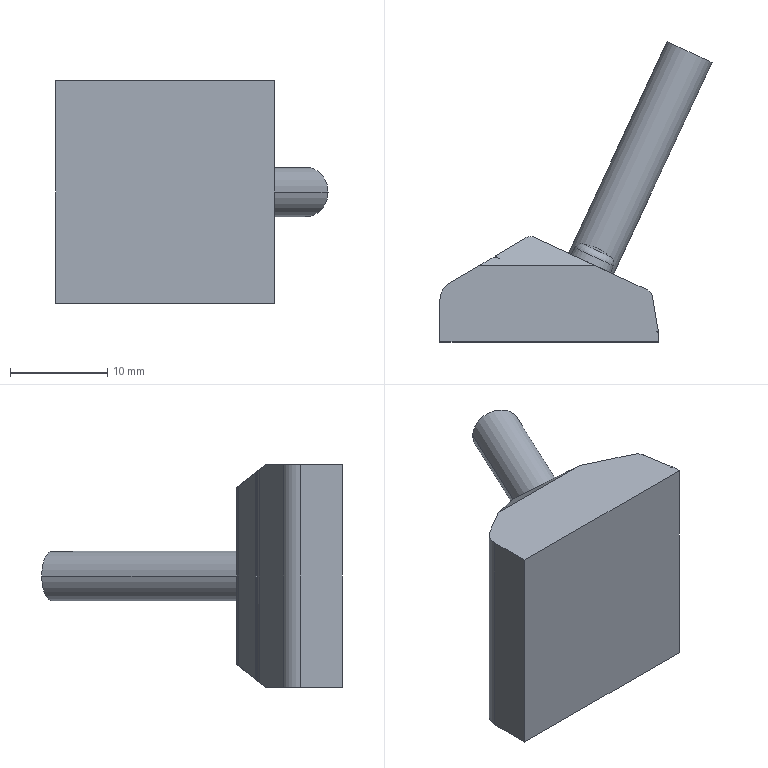Part | STEP file | Cable_Brake_Top_03_CE02_MSMF | 1 solid | 37 faces | box 27.962 x 30.887 x 22.9 mm | volume 4595 mm3 | plane 15 | cylinder 10 | cone 4 | torus 4 | other 4 | commonest cylinder face diameters 2 x4 0.2 x3 5.1 x2 4 x1